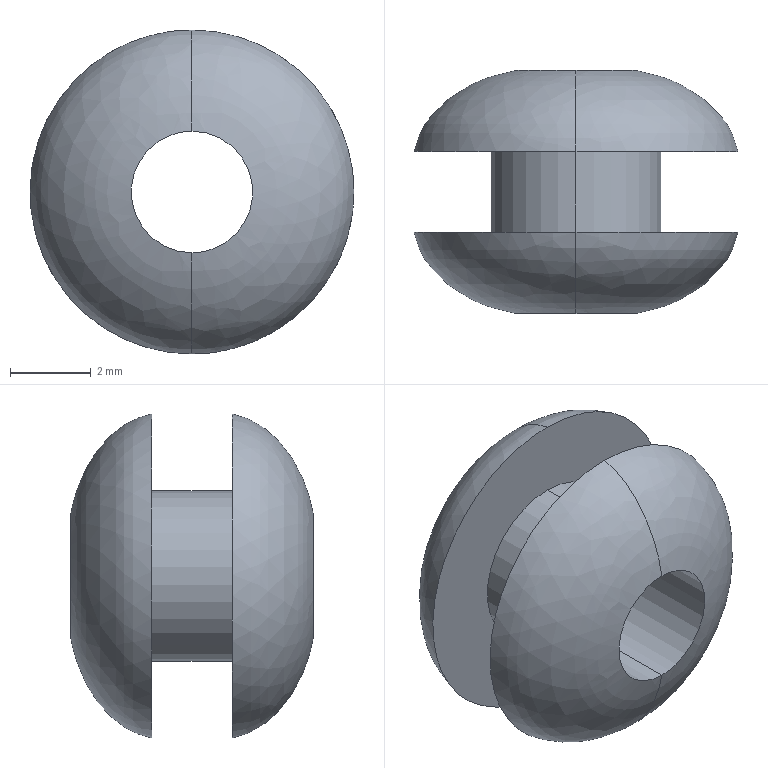Part | SolidWorks | features BaseBody 1 | 1 solid | 10 faces | box 8 x 6 x 8 mm | volume 125.45 mm3 | spline 4 | cylinder 4 | plane 2 | commonest cylinder face diameters 3 x2 4.2 x2
STEP:
#1=CARTESIAN_POINT('',(0.,-1.,-4.));
#2=VERTEX_POINT('',#1);
#3=CARTESIAN_POINT('',(0.,-3.,-1.5));
#4=VERTEX_POINT('',#3);
#5=CARTESIAN_POINT('',(0.,-1.,-4.));
#6=CARTESIAN_POINT('',(0.,-2.617,-3.692));
#7=CARTESIAN_POINT('',(0.,-3.,-1.5));
#8=(BOUNDED_CURVE()B_SPLINE_CURVE(2,(#5,#6,#7),.UNSPECIFIED.,.F.,.F.)B_SPLINE_CURVE_WITH_KNOTS((3,3),(0.,1.),.UNSPECIFIED.)CURVE()GEOMETRIC_REPRESENTATION_ITEM()RATIONAL_B_SPLINE_CURVE((1.,0.8226,1.))REPRESENTATION_ITEM(''));
#9=EDGE_CURVE('',#2,#4,#8,.T.);
#10=ORIENTED_EDGE('',*,*,#9,.F.);
#11=CARTESIAN_POINT('',(0.,-1.,4.));
#12=VERTEX_POINT('',#11);
#13=CARTESIAN_POINT('',(0.,-1.,4.));
#14=CARTESIAN_POINT('',(0.5299,-1.,4.));
#15=CARTESIAN_POINT('',(1.042,-1.,3.898));
#16=CARTESIAN_POINT('',(2.02,-1.,3.493));
#17=CARTESIAN_POINT('',(2.454,-1.,3.203));
#18=CARTESIAN_POINT('',(3.203,-1.,2.454));
#19=CARTESIAN_POINT('',(3.493,-1.,2.02));
#20=CARTESIAN_POINT('',(3.898,-1.,1.042));
#21=CARTESIAN_POINT('',(4.,-1.,0.5294));
#22=CARTESIAN_POINT('',(4.,-1.,-0.5294));
#23=CARTESIAN_POINT('',(3.898,-1.,-1.042));
#24=CARTESIAN_POINT('',(3.493,-1.,-2.02));
#25=CARTESIAN_POINT('',(3.203,-1.,-2.454));
#26=CARTESIAN_POINT('',(2.454,-1.,-3.203));
#27=CARTESIAN_POINT('',(2.02,-1.,-3.493));
#28=CARTESIAN_POINT('',(1.041,-1.,-3.898));
#29=CARTESIAN_POINT('',(0.5312,-1.,-4.));
#30=CARTESIAN_POINT('',(0.,-1.,-4.));
#31=B_SPLINE_CURVE_WITH_KNOTS('',3,(#13,#14,#15,#16,#17,#18,#19,#20,#21,#22,#23,#24,#25,#26,#27,#28,#29,#30),.UNSPECIFIED.,.F.,.F.,(4,2,2,2,2,2,2,2,4),(0.,0.125,0.25,0.375,0.5,0.625,0.75,0.875,1.),.UNSPECIFIED.);
#32=EDGE_CURVE('',#12,#2,#31,.T.);
#33=ORIENTED_EDGE('',*,*,#32,.F.);
#34=CARTESIAN_POINT('',(0.,-3.,1.5));
#35=VERTEX_POINT('',#34);
#36=CARTESIAN_POINT('',(0.,-1.,4.));
#37=CARTESIAN_POINT('',(0.,-2.617,3.692));
#38=CARTESIAN_POINT('',(0.,-3.,1.5));
#39=(BOUNDED_CURVE()B_SPLINE_CURVE(2,(#36,#37,#38),.UNSPECIFIED.,.F.,.F.)B_SPLINE_CURVE_WITH_KNOTS((3,3),(0.,1.),.UNSPECIFIED.)CURVE()GEOMETRIC_REPRESENTATION_ITEM()RATIONAL_B_SPLINE_CURVE((1.,0.8226,1.))REPRESENTATION_ITEM(''));
#40=EDGE_CURVE('',#12,#35,#39,.T.);
#41=ORIENTED_EDGE('',*,*,#40,.T.);
#42=CARTESIAN_POINT('',(0.,-3.,1.5));
#43=CARTESIAN_POINT('',(0.1963,-3.,1.5));
#44=CARTESIAN_POINT('',(0.3926,-3.,1.461));
#45=CARTESIAN_POINT('',(0.7554,-3.,1.311));
#46=CARTESIAN_POINT('',(0.9218,-3.,1.2));
#47=CARTESIAN_POINT('',(1.2,-3.,0.9218));
#48=CARTESIAN_POINT('',(1.311,-3.,0.7554));
#49=CARTESIAN_POINT('',(1.461,-3.,0.3926));
#50=CARTESIAN_POINT('',(1.5,-3.,0.1963));
#51=CARTESIAN_POINT('',(1.5,-3.,-0.1963));
#52=CARTESIAN_POINT('',(1.461,-3.,-0.3926));
#53=CARTESIAN_POINT('',(1.311,-3.,-0.7554));
#54=CARTESIAN_POINT('',(1.2,-3.,-0.9218));
#55=CARTESIAN_POINT('',(0.9218,-3.,-1.2));
#56=CARTESIAN_POINT('',(0.7554,-3.,-1.311));
#57=CARTESIAN_POINT('',(0.3926,-3.,-1.461));
#58=CARTESIAN_POINT('',(0.1963,-3.,-1.5));
#59=CARTESIAN_POINT('',(0.,-3.,-1.5));
#60=B_SPLINE_CURVE_WITH_KNOTS('',3,(#42,#43,#44,#45,#46,#47,#48,#49,#50,#51,#52,#53,#54,#55,#56,#57,#58,#59),.UNSPECIFIED.,.F.,.F.,(4,2,2,2,2,2,2,2,4),(0.,0.125,0.25,0.375,0.5,0.625,0.75,0.875,1.),.UNSPECIFIED.);
#61=EDGE_CURVE('',#35,#4,#60,.T.);
#62=ORIENTED_EDGE('',*,*,#61,.T.);
#63=EDGE_LOOP('',(#10,#33,#41,#62));
#64=FACE_OUTER_BOUND('',#63,.T.);
#65=CARTESIAN_POINT('',(0.,-1.,4.));
#66=CARTESIAN_POINT('',(0.5236,-1.,4.));
#67=CARTESIAN_POINT('',(1.047,-1.,3.896));
#68=CARTESIAN_POINT('',(2.014,-1.,3.495));
#69=CARTESIAN_POINT('',(2.458,-1.,3.199));
#70=CARTESIAN_POINT('',(3.199,-1.,2.458));
#71=CARTESIAN_POINT('',(3.495,-1.,2.014));
#72=CARTESIAN_POINT('',(3.896,-1.,1.047));
#73=CARTESIAN_POINT('',(4.,-1.,0.5236));
#74=CARTESIAN_POINT('',(4.,-1.,-0.5236));
#75=CARTESIAN_POINT('',(3.896,-1.,-1.047));
#76=CARTESIAN_POINT('',(3.495,-1.,-2.014));
#77=CARTESIAN_POINT('',(3.199,-1.,-2.458));
#78=CARTESIAN_POINT('',(2.458,-1.,-3.199));
#79=CARTESIAN_POINT('',(2.014,-1.,-3.495));
#80=CARTESIAN_POINT('',(1.047,-1.,-3.896));
#81=CARTESIAN_POINT('',(0.5236,-1.,-4.));
#82=CARTESIAN_POINT('',(-0.5236,-1.,-4.));
#83=CARTESIAN_POINT('',(-1.047,-1.,-3.896));
#84=CARTESIAN_POINT('',(-2.014,-1.,-3.495));
#85=CARTESIAN_POINT('',(-2.458,-1.,-3.199));
#86=CARTESIAN_POINT('',(-3.199,-1.,-2.458));
#87=CARTESIAN_POINT('',(-3.495,-1.,-2.014));
#88=CARTESIAN_POINT('',(-3.896,-1.,-1.047));
#89=CARTESIAN_POINT('',(-4.,-1.,-0.5236));
#90=CARTESIAN_POINT('',(-4.,-1.,0.5236));
#91=CARTESIAN_POINT('',(-3.896,-1.,1.047));
#92=CARTESIAN_POINT('',(-3.495,-1.,2.014));
#93=CARTESIAN_POINT('',(-3.199,-1.,2.458));
#94=CARTESIAN_POINT('',(-2.458,-1.,3.199));
#95=CARTESIAN_POINT('',(-2.014,-1.,3.495));
#96=CARTESIAN_POINT('',(-1.047,-1.,3.896));
#97=CARTESIAN_POINT('',(-0.5236,-1.,4.));
#98=CARTESIAN_POINT('',(0.,-1.,4.));
#99=CARTESIAN_POINT('',(0.,-2.617,3.692));
#100=CARTESIAN_POINT('',(0.4833,-2.617,3.692));
#101=CARTESIAN_POINT('',(0.9664,-2.617,3.596));
#102=CARTESIAN_POINT('',(1.859,-2.617,3.226));
#103=CARTESIAN_POINT('',(2.269,-2.617,2.952));
#104=CARTESIAN_POINT('',(2.952,-2.617,2.269));
#105=CARTESIAN_POINT('',(3.226,-2.617,1.859));
#106=CARTESIAN_POINT('',(3.596,-2.617,0.9664));
#107=CARTESIAN_POINT('',(3.692,-2.617,0.4833));
#108=CARTESIAN_POINT('',(3.692,-2.617,-0.4833));
#109=CARTESIAN_POINT('',(3.596,-2.617,-0.9664));
#110=CARTESIAN_POINT('',(3.226,-2.617,-1.859));
#111=CARTESIAN_POINT('',(2.952,-2.617,-2.269));
#112=CARTESIAN_POINT('',(2.269,-2.617,-2.952));
#113=CARTESIAN_POINT('',(1.859,-2.617,-3.226));
#114=CARTESIAN_POINT('',(0.9664,-2.617,-3.596));
#115=CARTESIAN_POINT('',(0.4833,-2.617,-3.692));
#116=CARTESIAN_POINT('',(-0.4833,-2.617,-3.692));
#117=CARTESIAN_POINT('',(-0.9664,-2.617,-3.596));
#118=CARTESIAN_POINT('',(-1.859,-2.617,-3.226));
#119=CARTESIAN_POINT('',(-2.269,-2.617,-2.952));
#120=CARTESIAN_POINT('',(-2.952,-2.617,-2.269));
#121=CARTESIAN_POINT('',(-3.226,-2.617,-1.859));
#122=CARTESIAN_POINT('',(-3.596,-2.617,-0.9664));
#123=CARTESIAN_POINT('',(-3.692,-2.617,-0.4833));
#124=CARTESIAN_POINT('',(-3.692,-2.617,0.4833));
#125=CARTESIAN_POINT('',(-3.596,-2.617,0.9664));
#126=CARTESIAN_POINT('',(-3.226,-2.617,1.859));
#127=CARTESIAN_POINT('',(-2.952,-2.617,2.269));
#128=CARTESIAN_POINT('',(-2.269,-2.617,2.952));
#129=CARTESIAN_POINT('',(-1.859,-2.617,3.226));
#130=CARTESIAN_POINT('',(-0.9664,-2.617,3.596));
#131=CARTESIAN_POINT('',(-0.4833,-2.617,3.692));
#132=CARTESIAN_POINT('',(0.,-2.617,3.692));
#133=CARTESIAN_POINT('',(0.,-3.,1.5));
#134=CARTESIAN_POINT('',(0.1963,-3.,1.5));
#135=CARTESIAN_POINT('',(0.3926,-3.,1.461));
#136=CARTESIAN_POINT('',(0.7554,-3.,1.311));
#137=CARTESIAN_POINT('',(0.9218,-3.,1.2));
#138=CARTESIAN_POINT('',(1.2,-3.,0.9218));
#139=CARTESIAN_POINT('',(1.311,-3.,0.7554));
#140=CARTESIAN_POINT('',(1.461,-3.,0.3926));
#141=CARTESIAN_POINT('',(1.5,-3.,0.1963));
#142=CARTESIAN_POINT('',(1.5,-3.,-0.1963));
#143=CARTESIAN_POINT('',(1.461,-3.,-0.3926));
#144=CARTESIAN_POINT('',(1.311,-3.,-0.7554));
#145=CARTESIAN_POINT('',(1.2,-3.,-0.9218));
#146=CARTESIAN_POINT('',(0.9218,-3.,-1.2));
#147=CARTESIAN_POINT('',(0.7554,-3.,-1.311));
#148=CARTESIAN_POINT('',(0.3926,-3.,-1.461));
#149=CARTESIAN_POINT('',(0.1963,-3.,-1.5));
#150=CARTESIAN_POINT('',(-0.1963,-3.,-1.5));
#151=CARTESIAN_POINT('',(-0.3926,-3.,-1.461));
#152=CARTESIAN_POINT('',(-0.7554,-3.,-1.311));
#153=CARTESIAN_POINT('',(-0.9218,-3.,-1.2));
#154=CARTESIAN_POINT('',(-1.2,-3.,-0.9218));
#155=CARTESIAN_POINT('',(-1.311,-3.,-0.7554));
#156=CARTESIAN_POINT('',(-1.461,-3.,-0.3926));
#157=CARTESIAN_POINT('',(-1.5,-3.,-0.1963));
#158=CARTESIAN_POINT('',(-1.5,-3.,0.1963));
#159=CARTESIAN_POINT('',(-1.461,-3.,0.3926));
#160=CARTESIAN_POINT('',(-1.311,-3.,0.7554));
#161=CARTESIAN_POINT('',(-1.2,-3.,0.9218));
#162=CARTESIAN_POINT('',(-0.9218,-3.,1.2));
#163=CARTESIAN_POINT('',(-0.7554,-3.,1.311));
#164=CARTESIAN_POINT('',(-0.3926,-3.,1.461));
#165=CARTESIAN_POINT('',(-0.1963,-3.,1.5));
#166=CARTESIAN_POINT('',(0.,-3.,1.5));
#167=(BOUNDED_SURFACE()B_SPLINE_SURFACE(2,3,((#65,#66,#67,#68,#69,#70,#71,#72,#73,#74,#75,#76,#77,#78,#79,#80,#81,#82,#83,#84,#85,#86,#87,#88,#89,#90,#91,#92,#93,#94,#95,#96,#97,#98),(#99,#100,#101,#102,#103,#104,#105,#106,#107,#108,#109,#110,#111,#112,#113,#114,#115,#116,#117,#118,#119,#120,#121,#122,#123,#124,#125,#126,#127,#128,#129,#130,#131,#132),(#133,#134,#135,#136,#137,#138,#139,#140,#141,#142,#143,#144,#145,#146,#147,#148,#149,#150,#151,#152,#153,#154,#155,#156,#157,#158,#159,#160,#161,#162,#163,#164,#165,#166)),.UNSPECIFIED.,.F.,.T.,.F.)B_SPLINE_SURFACE_WITH_KNOTS((3,3),(4,2,2,2,2,2,2,2,2,2,2,2,2,2,2,2,4),(0.,1.),(0.,0.3927,0.7854,1.178,1.571,1.963,2.356,2.749,3.142,3.534,3.927,4.32,4.712,5.105,5.498,5.89,6.283),.UNSPECIFIED.)GEOMETRIC_REPRESENTATION_ITEM()RATIONAL_B_SPLINE_SURFACE(((1.,1.,1.,1.,1.,1.,1.,1.,1.,1.,1.,1.,1.,1.,1.,1.,1.,1.,1.,1.,1.,1.,1.,1.,1.,1.,1.,1.,1.,1.,1.,1.,1.,1.),(0.8226,0.8226,0.8226,0.8226,0.8226,0.8226,0.8226,0.8226,0.8226,0.8226,0.8226,0.8226,0.8226,0.8226,0.8226,0.8226,0.8226,0.8226,0.8226,0.8226,0.8226,0.8226,0.8226,0.8226,0.8226,0.8226,0.8226,0.8226,0.8226,0.8226,0.8226,0.8226,0.8226,0.8226),(1.,1.,1.,1.,1.,1.,1.,1.,1.,1.,1.,1.,1.,1.,1.,1.,1.,1.,1.,1.,1.,1.,1.,1.,1.,1.,1.,1.,1.,1.,1.,1.,1.,1.)))REPRESENTATION_ITEM('')SURFACE());
#168=ADVANCED_FACE('',(#64),#167,.T.);
#169=CARTESIAN_POINT('',(0.,-1.,-2.1));
#170=VERTEX_POINT('',#169);
#171=CARTESIAN_POINT('',(0.,-1.,2.1));
#172=VERTEX_POINT('',#171);
#173=CARTESIAN_POINT('',(0.,-1.,0.));
#174=DIRECTION('',(0.,1.,0.));
#175=DIRECTION('',(0.,0.,1.));
#176=AXIS2_PLACEMENT_3D('',#173,#174,#175);
#177=CIRCLE('',#176,2.1);
#178=EDGE_CURVE('',#170,#172,#177,.T.);
#179=ORIENTED_EDGE('',*,*,#178,.F.);
#180=CARTESIAN_POINT('',(0.,-1.,0.));
#181=DIRECTION('',(0.,1.,0.));
#182=DIRECTION('',(0.,0.,1.));
#183=AXIS2_PLACEMENT_3D('',#180,#181,#182);
#184=CIRCLE('',#183,2.1);
#185=EDGE_CURVE('',#172,#170,#184,.T.);
#186=ORIENTED_EDGE('',*,*,#185,.F.);
#187=EDGE_LOOP('',(#179,#186));
#188=FACE_BOUND('',#187,.T.);
#189=ORIENTED_EDGE('',*,*,#32,.T.);
#190=CARTESIAN_POINT('',(0.,-1.,-4.));
#191=CARTESIAN_POINT('',(-0.5297,-1.,-4.));
#192=CARTESIAN_POINT('',(-1.042,-1.,-3.898));
#193=CARTESIAN_POINT('',(-2.02,-1.,-3.493));
#194=CARTESIAN_POINT('',(-2.454,-1.,-3.203));
#195=CARTESIAN_POINT('',(-3.203,-1.,-2.454));
#196=CARTESIAN_POINT('',(-3.493,-1.,-2.02));
#197=CARTESIAN_POINT('',(-3.898,-1.,-1.042));
#198=CARTESIAN_POINT('',(-4.,-1.,-0.5293));
#199=CARTESIAN_POINT('',(-4.,-1.,0.5293));
#200=CARTESIAN_POINT('',(-3.898,-1.,1.042));
#201=CARTESIAN_POINT('',(-3.493,-1.,2.02));
#202=CARTESIAN_POINT('',(-3.203,-1.,2.454));
#203=CARTESIAN_POINT('',(-2.454,-1.,3.203));
#204=CARTESIAN_POINT('',(-2.02,-1.,3.493));
#205=CARTESIAN_POINT('',(-1.041,-1.,3.899));
#206=CARTESIAN_POINT('',(-0.531,-1.,4.));
#207=CARTESIAN_POINT('',(0.,-1.,4.));
#208=B_SPLINE_CURVE_WITH_KNOTS('',3,(#190,#191,#192,#193,#194,#195,#196,#197,#198,#199,#200,#201,#202,#203,#204,#205,#206,#207),.UNSPECIFIED.,.F.,.F.,(4,2,2,2,2,2,2,2,4),(0.,0.125,0.25,0.375,0.5,0.625,0.75,0.875,1.),.UNSPECIFIED.);
#209=EDGE_CURVE('',#2,#12,#208,.T.);
#210=ORIENTED_EDGE('',*,*,#209,.T.);
#211=EDGE_LOOP('',(#189,#210));
#212=FACE_OUTER_BOUND('',#211,.T.);
#213=CARTESIAN_POINT('',(0.,-1.,0.));
#214=DIRECTION('',(0.,-1.,0.));
#215=DIRECTION('',(0.,0.,-1.));
#216=AXIS2_PLACEMENT_3D('',#213,#214,#215);
#217=PLANE('',#216);
#218=ADVANCED_FACE('',(#188,#212),#217,.F.);
#219=CARTESIAN_POINT('',(0.,3.,-1.5));
#220=VERTEX_POINT('',#219);
#221=CARTESIAN_POINT('',(0.,1.,-4.));
#222=VERTEX_POINT('',#221);
#223=CARTESIAN_POINT('',(0.,3.,-1.5));
#224=CARTESIAN_POINT('',(0.,2.617,-3.692));
#225=CARTESIAN_POINT('',(0.,1.,-4.));
#226=(BOUNDED_CURVE()B_SPLINE_CURVE(2,(#223,#224,#225),.UNSPECIFIED.,.F.,.F.)B_SPLINE_CURVE_WITH_KNOTS((3,3),(0.,1.),.UNSPECIFIED.)CURVE()GEOMETRIC_REPRESENTATION_ITEM()RATIONAL_B_SPLINE_CURVE((1.,0.8226,1.))REPRESENTATION_ITEM(''));
#227=EDGE_CURVE('',#220,#222,#226,.T.);
#228=ORIENTED_EDGE('',*,*,#227,.F.);
#229=CARTESIAN_POINT('',(0.,3.,1.5));
#230=VERTEX_POINT('',#229);
#231=CARTESIAN_POINT('',(0.,3.,1.5));
#232=CARTESIAN_POINT('',(0.1963,3.,1.5));
#233=CARTESIAN_POINT('',(0.3926,3.,1.461));
#234=CARTESIAN_POINT('',(0.7554,3.,1.311));
#235=CARTESIAN_POINT('',(0.9218,3.,1.2));
#236=CARTESIAN_POINT('',(1.2,3.,0.9218));
#237=CARTESIAN_POINT('',(1.311,3.,0.7554));
#238=CARTESIAN_POINT('',(1.461,3.,0.3926));
#239=CARTESIAN_POINT('',(1.5,3.,0.1963));
#240=CARTESIAN_POINT('',(1.5,3.,-0.1963));
#241=CARTESIAN_POINT('',(1.461,3.,-0.3926));
#242=CARTESIAN_POINT('',(1.311,3.,-0.7554));
#243=CARTESIAN_POINT('',(1.2,3.,-0.9218));
#244=CARTESIAN_POINT('',(0.9218,3.,-1.2));
#245=CARTESIAN_POINT('',(0.7554,3.,-1.311));
#246=CARTESIAN_POINT('',(0.3926,3.,-1.461));
#247=CARTESIAN_POINT('',(0.1963,3.,-1.5));
#248=CARTESIAN_POINT('',(0.,3.,-1.5));
#249=B_SPLINE_CURVE_WITH_KNOTS('',3,(#231,#232,#233,#234,#235,#236,#237,#238,#239,#240,#241,#242,#243,#244,#245,#246,#247,#248),.UNSPECIFIED.,.F.,.F.,(4,2,2,2,2,2,2,2,4),(0.,0.125,0.25,0.375,0.5,0.625,0.75,0.875,1.),.UNSPECIFIED.);
#250=EDGE_CURVE('',#230,#220,#249,.T.);
#251=ORIENTED_EDGE('',*,*,#250,.F.);
#252=CARTESIAN_POINT('',(0.,1.,4.));
#253=VERTEX_POINT('',#252);
#254=CARTESIAN_POINT('',(0.,3.,1.5));
#255=CARTESIAN_POINT('',(0.,2.617,3.692));
#256=CARTESIAN_POINT('',(0.,1.,4.));
#257=(BOUNDED_CURVE()B_SPLINE_CURVE(2,(#254,#255,#256),.UNSPECIFIED.,.F.,.F.)B_SPLINE_CURVE_WITH_KNOTS((3,3),(0.,1.),.UNSPECIFIED.)CURVE()GEOMETRIC_REPRESENTATION_ITEM()RATIONAL_B_SPLINE_CURVE((1.,0.8226,1.))REPRESENTATION_ITEM(''));
#258=EDGE_CURVE('',#230,#253,#257,.T.);
#259=ORIENTED_EDGE('',*,*,#258,.T.);
#260=CARTESIAN_POINT('',(0.,1.,4.));
#261=CARTESIAN_POINT('',(0.5236,1.,4.));
#262=CARTESIAN_POINT('',(1.047,1.,3.896));
#263=CARTESIAN_POINT('',(2.014,1.,3.495));
#264=CARTESIAN_POINT('',(2.458,1.,3.199));
#265=CARTESIAN_POINT('',(3.199,1.,2.458));
#266=CARTESIAN_POINT('',(3.495,1.,2.014));
#267=CARTESIAN_POINT('',(3.896,1.,1.047));
#268=CARTESIAN_POINT('',(4.,1.,0.5236));
#269=CARTESIAN_POINT('',(4.,1.,-0.5236));
#270=CARTESIAN_POINT('',(3.896,1.,-1.047));
#271=CARTESIAN_POINT('',(3.495,1.,-2.014));
#272=CARTESIAN_POINT('',(3.199,1.,-2.458));
#273=CARTESIAN_POINT('',(2.458,1.,-3.199));
#274=CARTESIAN_POINT('',(2.014,1.,-3.495));
#275=CARTESIAN_POINT('',(1.047,1.,-3.896));
#276=CARTESIAN_POINT('',(0.5236,1.,-4.));
#277=CARTESIAN_POINT('',(0.,1.,-4.));
#278=B_SPLINE_CURVE_WITH_KNOTS('',3,(#260,#261,#262,#263,#264,#265,#266,#267,#268,#269,#270,#271,#272,#273,#274,#275,#276,#277),.UNSPECIFIED.,.F.,.F.,(4,2,2,2,2,2,2,2,4),(0.,0.0625,0.125,0.1875,0.25,0.3125,0.375,0.4375,0.5),.UNSPECIFIED.);
#279=EDGE_CURVE('',#253,#222,#278,.T.);
#280=ORIENTED_EDGE('',*,*,#279,.T.);
#281=EDGE_LOOP('',(#228,#251,#259,#280));
#282=FACE_OUTER_BOUND('',#281,.T.);
#283=CARTESIAN_POINT('',(0.,3.,1.5));
#284=CARTESIAN_POINT('',(0.1963,3.,1.5));
#285=CARTESIAN_POINT('',(0.3926,3.,1.461));
#286=CARTESIAN_POINT('',(0.7554,3.,1.311));
#287=CARTESIAN_POINT('',(0.9218,3.,1.2));
#288=CARTESIAN_POINT('',(1.2,3.,0.9218));
#289=CARTESIAN_POINT('',(1.311,3.,0.7554));
#290=CARTESIAN_POINT('',(1.461,3.,0.3926));
#291=CARTESIAN_POINT('',(1.5,3.,0.1963));
#292=CARTESIAN_POINT('',(1.5,3.,-0.1963));
#293=CARTESIAN_POINT('',(1.461,3.,-0.3926));
#294=CARTESIAN_POINT('',(1.311,3.,-0.7554));
#295=CARTESIAN_POINT('',(1.2,3.,-0.9218));
#296=CARTESIAN_POINT('',(0.9218,3.,-1.2));
#297=CARTESIAN_POINT('',(0.7554,3.,-1.311));
#298=CARTESIAN_POINT('',(0.3926,3.,-1.461));
#299=CARTESIAN_POINT('',(0.1963,3.,-1.5));
#300=CARTESIAN_POINT('',(0.,3.,-1.5));
#301=CARTESIAN_POINT('',(0.,2.617,3.692));
#302=CARTESIAN_POINT('',(0.4833,2.617,3.692));
#303=CARTESIAN_POINT('',(0.9664,2.617,3.596));
#304=CARTESIAN_POINT('',(1.859,2.617,3.226));
#305=CARTESIAN_POINT('',(2.269,2.617,2.952));
#306=CARTESIAN_POINT('',(2.952,2.617,2.269));
#307=CARTESIAN_POINT('',(3.226,2.617,1.859));
#308=CARTESIAN_POINT('',(3.596,2.617,0.9664));
#309=CARTESIAN_POINT('',(3.692,2.617,0.4833));
#310=CARTESIAN_POINT('',(3.692,2.617,-0.4833));
#311=CARTESIAN_POINT('',(3.596,2.617,-0.9664));
#312=CARTESIAN_POINT('',(3.226,2.617,-1.859));
#313=CARTESIAN_POINT('',(2.952,2.617,-2.269));
#314=CARTESIAN_POINT('',(2.269,2.617,-2.952));
#315=CARTESIAN_POINT('',(1.859,2.617,-3.226));
#316=CARTESIAN_POINT('',(0.9664,2.617,-3.596));
#317=CARTESIAN_POINT('',(0.4833,2.617,-3.692));
#318=CARTESIAN_POINT('',(0.,2.617,-3.692));
#319=CARTESIAN_POINT('',(0.,1.,4.));
#320=CARTESIAN_POINT('',(0.5236,1.,4.));
#321=CARTESIAN_POINT('',(1.047,1.,3.896));
#322=CARTESIAN_POINT('',(2.014,1.,3.495));
#323=CARTESIAN_POINT('',(2.458,1.,3.199));
#324=CARTESIAN_POINT('',(3.199,1.,2.458));
#325=CARTESIAN_POINT('',(3.495,1.,2.014));
#326=CARTESIAN_POINT('',(3.896,1.,1.047));
#327=CARTESIAN_POINT('',(4.,1.,0.5236));
#328=CARTESIAN_POINT('',(4.,1.,-0.5236));
#329=CARTESIAN_POINT('',(3.896,1.,-1.047));
#330=CARTESIAN_POINT('',(3.495,1.,-2.014));
#331=CARTESIAN_POINT('',(3.199,1.,-2.458));
#332=CARTESIAN_POINT('',(2.458,1.,-3.199));
#333=CARTESIAN_POINT('',(2.014,1.,-3.495));
#334=CARTESIAN_POINT('',(1.047,1.,-3.896));
#335=CARTESIAN_POINT('',(0.5236,1.,-4.));
#336=CARTESIAN_POINT('',(0.,1.,-4.));
#337=(BOUNDED_SURFACE()B_SPLINE_SURFACE(2,3,((#283,#284,#285,#286,#287,#288,#289,#290,#291,#292,#293,#294,#295,#296,#297,#298,#299,#300),(#301,#302,#303,#304,#305,#306,#307,#308,#309,#310,#311,#312,#313,#314,#315,#316,#317,#318),(#319,#320,#321,#322,#323,#324,#325,#326,#327,#328,#329,#330,#331,#332,#333,#334,#335,#336)),.UNSPECIFIED.,.F.,.F.,.T.)B_SPLINE_SURFACE_WITH_KNOTS((3,3),(4,2,2,2,2,2,2,2,4),(0.,1.),(0.,0.3927,0.7854,1.178,1.571,1.963,2.356,2.749,3.142),.UNSPECIFIED.)GEOMETRIC_REPRESENTATION_ITEM()RATIONAL_B_SPLINE_SURFACE(((1.,1.,1.,1.,1.,1.,1.,1.,1.,1.,1.,1.,1.,1.,1.,1.,1.,1.),(0.8226,0.8226,0.8226,0.8226,0.8226,0.8226,0.8226,0.8226,0.8226,0.8226,0.8226,0.8226,0.8226,0.8226,0.8226,0.8226,0.8226,0.8226),(1.,1.,1.,1.,1.,1.,1.,1.,1.,1.,1.,1.,1.,1.,1.,1.,1.,1.)))REPRESENTATION_ITEM('')SURFACE());
#338=ADVANCED_FACE('',(#282),#337,.T.);
#339=CARTESIAN_POINT('',(0.,1.,-2.1));
#340=VERTEX_POINT('',#339);
#341=CARTESIAN_POINT('',(0.,1.,2.1));
#342=VERTEX_POINT('',#341);
#343=CARTESIAN_POINT('',(0.,1.,0.));
#344=DIRECTION('',(0.,1.,0.));
#345=DIRECTION('',(0.,0.,1.));
#346=AXIS2_PLACEMENT_3D('',#343,#344,#345);
#347=CIRCLE('',#346,2.1);
#348=EDGE_CURVE('',#340,#342,#347,.T.);
#349=ORIENTED_EDGE('',*,*,#348,.T.);
#350=CARTESIAN_POINT('',(0.,1.,0.));
#351=DIRECTION('',(0.,1.,0.));
#352=DIRECTION('',(0.,0.,1.));
#353=AXIS2_PLACEMENT_3D('',#350,#351,#352);
#354=CIRCLE('',#353,2.1);
#355=EDGE_CURVE('',#342,#340,#354,.T.);
#356=ORIENTED_EDGE('',*,*,#355,.T.);
#357=EDGE_LOOP('',(#349,#356));
#358=FACE_BOUND('',#357,.T.);
#359=ORIENTED_EDGE('',*,*,#279,.F.);
#360=CARTESIAN_POINT('',(0.,1.,-4.));
#361=CARTESIAN_POINT('',(-0.5236,1.,-4.));
#362=CARTESIAN_POINT('',(-1.047,1.,-3.896));
#363=CARTESIAN_POINT('',(-2.014,1.,-3.495));
#364=CARTESIAN_POINT('',(-2.458,1.,-3.199));
#365=CARTESIAN_POINT('',(-3.199,1.,-2.458));
#366=CARTESIAN_POINT('',(-3.495,1.,-2.014));
#367=CARTESIAN_POINT('',(-3.896,1.,-1.047));
#368=CARTESIAN_POINT('',(-4.,1.,-0.5236));
#369=CARTESIAN_POINT('',(-4.,1.,0.5236));
#370=CARTESIAN_POINT('',(-3.896,1.,1.047));
#371=CARTESIAN_POINT('',(-3.495,1.,2.014));
#372=CARTESIAN_POINT('',(-3.199,1.,2.458));
#373=CARTESIAN_POINT('',(-2.458,1.,3.199));
#374=CARTESIAN_POINT('',(-2.014,1.,3.495));
#375=CARTESIAN_POINT('',(-1.047,1.,3.896));
#376=CARTESIAN_POINT('',(-0.5236,1.,4.));
#377=CARTESIAN_POINT('',(0.,1.,4.));
#378=B_SPLINE_CURVE_WITH_KNOTS('',3,(#360,#361,#362,#363,#364,#365,#366,#367,#368,#369,#370,#371,#372,#373,#374,#375,#376,#377),.UNSPECIFIED.,.F.,.F.,(4,2,2,2,2,2,2,2,4),(0.5,0.5625,0.625,0.6875,0.75,0.8125,0.875,0.9375,1.),.UNSPECIFIED.);
#379=EDGE_CURVE('',#222,#253,#378,.T.);
#380=ORIENTED_EDGE('',*,*,#379,.F.);
#381=EDGE_LOOP('',(#359,#380));
#382=FACE_OUTER_BOUND('',#381,.T.);
#383=CARTESIAN_POINT('',(0.,1.,0.));
#384=DIRECTION('',(0.,1.,0.));
#385=DIRECTION('',(1.,0.,0.));
#386=AXIS2_PLACEMENT_3D('',#383,#384,#385);
#387=PLANE('',#386);
#388=ADVANCED_FACE('',(#358,#382),#387,.F.);
#389=CARTESIAN_POINT('',(0.,1.,1.5));
#390=DIRECTION('',(0.,-1.,0.));
#391=VECTOR('',#390,1000.);
#392=LINE('',#389,#391);
#393=EDGE_CURVE('',#230,#35,#392,.T.);
#394=ORIENTED_EDGE('',*,*,#393,.F.);
#395=ORIENTED_EDGE('',*,*,#250,.T.);
#396=CARTESIAN_POINT('',(0.,1.,-1.5));
#397=DIRECTION('',(0.,-1.,0.));
#398=VECTOR('',#397,1000.);
#399=LINE('',#396,#398);
#400=EDGE_CURVE('',#220,#4,#399,.T.);
#401=ORIENTED_EDGE('',*,*,#400,.T.);
#402=ORIENTED_EDGE('',*,*,#61,.F.);
#403=EDGE_LOOP('',(#394,#395,#401,#402));
#404=FACE_OUTER_BOUND('',#403,.T.);
#405=CARTESIAN_POINT('',(0.,1.,0.));
#406=DIRECTION('',(0.,-1.,0.));
#407=DIRECTION('',(0.,0.,-1.));
#408=AXIS2_PLACEMENT_3D('',#405,#406,#407);
#409=CYLINDRICAL_SURFACE('',#408,1.5);
#410=ADVANCED_FACE('',(#404),#409,.F.);
#411=CARTESIAN_POINT('',(0.,1.,2.1));
#412=DIRECTION('',(0.,-1.,0.));
#413=VECTOR('',#412,1000.);
#414=LINE('',#411,#413);
#415=EDGE_CURVE('',#342,#172,#414,.T.);
#416=ORIENTED_EDGE('',*,*,#415,.F.);
#417=ORIENTED_EDGE('',*,*,#348,.F.);
#418=CARTESIAN_POINT('',(0.,1.,-2.1));
#419=DIRECTION('',(0.,-1.,0.));
#420=VECTOR('',#419,1000.);
#421=LINE('',#418,#420);
#422=EDGE_CURVE('',#340,#170,#421,.T.);
#423=ORIENTED_EDGE('',*,*,#422,.T.);
#424=ORIENTED_EDGE('',*,*,#178,.T.);
#425=EDGE_LOOP('',(#416,#417,#423,#424));
#426=FACE_OUTER_BOUND('',#425,.T.);
#427=CARTESIAN_POINT('',(0.,1.,0.));
#428=DIRECTION('',(0.,-1.,0.));
#429=DIRECTION('',(0.,0.,-1.));
#430=AXIS2_PLACEMENT_3D('',#427,#428,#429);
#431=CYLINDRICAL_SURFACE('',#430,2.1);
#432=ADVANCED_FACE('',(#426),#431,.T.);
#433=ORIENTED_EDGE('',*,*,#355,.F.);
#434=ORIENTED_EDGE('',*,*,#415,.T.);
#435=ORIENTED_EDGE('',*,*,#185,.T.);
#436=ORIENTED_EDGE('',*,*,#422,.F.);
#437=EDGE_LOOP('',(#433,#434,#435,#436));
#438=FACE_OUTER_BOUND('',#437,.T.);
#439=CARTESIAN_POINT('',(0.,1.,0.));
#440=DIRECTION('',(0.,-1.,0.));
#441=DIRECTION('',(0.,0.,-1.));
#442=AXIS2_PLACEMENT_3D('',#439,#440,#441);
#443=CYLINDRICAL_SURFACE('',#442,2.1);
#444=ADVANCED_FACE('',(#438),#443,.T.);
#445=CARTESIAN_POINT('',(0.,3.,-1.5));
#446=CARTESIAN_POINT('',(-0.1963,3.,-1.5));
#447=CARTESIAN_POINT('',(-0.3926,3.,-1.461));
#448=CARTESIAN_POINT('',(-0.7554,3.,-1.311));
#449=CARTESIAN_POINT('',(-0.9218,3.,-1.2));
#450=CARTESIAN_POINT('',(-1.2,3.,-0.9218));
#451=CARTESIAN_POINT('',(-1.311,3.,-0.7554));
#452=CARTESIAN_POINT('',(-1.461,3.,-0.3926));
#453=CARTESIAN_POINT('',(-1.5,3.,-0.1963));
#454=CARTESIAN_POINT('',(-1.5,3.,0.1963));
#455=CARTESIAN_POINT('',(-1.461,3.,0.3926));
#456=CARTESIAN_POINT('',(-1.311,3.,0.7554));
#457=CARTESIAN_POINT('',(-1.2,3.,0.9218));
#458=CARTESIAN_POINT('',(-0.9218,3.,1.2));
#459=CARTESIAN_POINT('',(-0.7554,3.,1.311));
#460=CARTESIAN_POINT('',(-0.3926,3.,1.461));
#461=CARTESIAN_POINT('',(-0.1963,3.,1.5));
#462=CARTESIAN_POINT('',(0.,3.,1.5));
#463=B_SPLINE_CURVE_WITH_KNOTS('',3,(#445,#446,#447,#448,#449,#450,#451,#452,#453,#454,#455,#456,#457,#458,#459,#460,#461,#462),.UNSPECIFIED.,.F.,.F.,(4,2,2,2,2,2,2,2,4),(0.,0.125,0.25,0.375,0.5,0.625,0.75,0.875,1.),.UNSPECIFIED.);
#464=EDGE_CURVE('',#220,#230,#463,.T.);
#465=ORIENTED_EDGE('',*,*,#464,.T.);
#466=ORIENTED_EDGE('',*,*,#393,.T.);
#467=CARTESIAN_POINT('',(0.,-3.,-1.5));
#468=CARTESIAN_POINT('',(-0.1963,-3.,-1.5));
#469=CARTESIAN_POINT('',(-0.3926,-3.,-1.461));
#470=CARTESIAN_POINT('',(-0.7554,-3.,-1.311));
#471=CARTESIAN_POINT('',(-0.9218,-3.,-1.2));
#472=CARTESIAN_POINT('',(-1.2,-3.,-0.9218));
#473=CARTESIAN_POINT('',(-1.311,-3.,-0.7554));
#474=CARTESIAN_POINT('',(-1.461,-3.,-0.3926));
#475=CARTESIAN_POINT('',(-1.5,-3.,-0.1963));
#476=CARTESIAN_POINT('',(-1.5,-3.,0.1963));
#477=CARTESIAN_POINT('',(-1.461,-3.,0.3926));
#478=CARTESIAN_POINT('',(-1.311,-3.,0.7554));
#479=CARTESIAN_POINT('',(-1.2,-3.,0.9218));
#480=CARTESIAN_POINT('',(-0.9218,-3.,1.2));
#481=CARTESIAN_POINT('',(-0.7554,-3.,1.311));
#482=CARTESIAN_POINT('',(-0.3926,-3.,1.461));
#483=CARTESIAN_POINT('',(-0.1963,-3.,1.5));
#484=CARTESIAN_POINT('',(0.,-3.,1.5));
#485=B_SPLINE_CURVE_WITH_KNOTS('',3,(#467,#468,#469,#470,#471,#472,#473,#474,#475,#476,#477,#478,#479,#480,#481,#482,#483,#484),.UNSPECIFIED.,.F.,.F.,(4,2,2,2,2,2,2,2,4),(0.,0.125,0.25,0.375,0.5,0.625,0.75,0.875,1.),.UNSPECIFIED.);
#486=EDGE_CURVE('',#4,#35,#485,.T.);
#487=ORIENTED_EDGE('',*,*,#486,.F.);
#488=ORIENTED_EDGE('',*,*,#400,.F.);
#489=EDGE_LOOP('',(#465,#466,#487,#488));
#490=FACE_OUTER_BOUND('',#489,.T.);
#491=CARTESIAN_POINT('',(0.,1.,0.));
#492=DIRECTION('',(0.,-1.,0.));
#493=DIRECTION('',(0.,0.,-1.));
#494=AXIS2_PLACEMENT_3D('',#491,#492,#493);
#495=CYLINDRICAL_SURFACE('',#494,1.5);
#496=ADVANCED_FACE('',(#490),#495,.F.);
#497=ORIENTED_EDGE('',*,*,#464,.F.);
#498=ORIENTED_EDGE('',*,*,#227,.T.);
#499=ORIENTED_EDGE('',*,*,#379,.T.);
#500=ORIENTED_EDGE('',*,*,#258,.F.);
#501=EDGE_LOOP('',(#497,#498,#499,#500));
#502=FACE_OUTER_BOUND('',#501,.T.);
#503=CARTESIAN_POINT('',(0.,3.,-1.5));
#504=CARTESIAN_POINT('',(-0.1963,3.,-1.5));
#505=CARTESIAN_POINT('',(-0.3926,3.,-1.461));
#506=CARTESIAN_POINT('',(-0.7554,3.,-1.311));
#507=CARTESIAN_POINT('',(-0.9218,3.,-1.2));
#508=CARTESIAN_POINT('',(-1.2,3.,-0.9218));
#509=CARTESIAN_POINT('',(-1.311,3.,-0.7554));
#510=CARTESIAN_POINT('',(-1.461,3.,-0.3926));
#511=CARTESIAN_POINT('',(-1.5,3.,-0.1963));
#512=CARTESIAN_POINT('',(-1.5,3.,0.1963));
#513=CARTESIAN_POINT('',(-1.461,3.,0.3926));
#514=CARTESIAN_POINT('',(-1.311,3.,0.7554));
#515=CARTESIAN_POINT('',(-1.2,3.,0.9218));
#516=CARTESIAN_POINT('',(-0.9218,3.,1.2));
#517=CARTESIAN_POINT('',(-0.7554,3.,1.311));
#518=CARTESIAN_POINT('',(-0.3926,3.,1.461));
#519=CARTESIAN_POINT('',(-0.1963,3.,1.5));
#520=CARTESIAN_POINT('',(0.,3.,1.5));
#521=CARTESIAN_POINT('',(0.,2.617,-3.692));
#522=CARTESIAN_POINT('',(-0.4833,2.617,-3.692));
#523=CARTESIAN_POINT('',(-0.9664,2.617,-3.596));
#524=CARTESIAN_POINT('',(-1.859,2.617,-3.226));
#525=CARTESIAN_POINT('',(-2.269,2.617,-2.952));
#526=CARTESIAN_POINT('',(-2.952,2.617,-2.269));
#527=CARTESIAN_POINT('',(-3.226,2.617,-1.859));
#528=CARTESIAN_POINT('',(-3.596,2.617,-0.9664));
#529=CARTESIAN_POINT('',(-3.692,2.617,-0.4833));
#530=CARTESIAN_POINT('',(-3.692,2.617,0.4833));
#531=CARTESIAN_POINT('',(-3.596,2.617,0.9664));
#532=CARTESIAN_POINT('',(-3.226,2.617,1.859));
#533=CARTESIAN_POINT('',(-2.952,2.617,2.269));
#534=CARTESIAN_POINT('',(-2.269,2.617,2.952));
#535=CARTESIAN_POINT('',(-1.859,2.617,3.226));
#536=CARTESIAN_POINT('',(-0.9664,2.617,3.596));
#537=CARTESIAN_POINT('',(-0.4833,2.617,3.692));
#538=CARTESIAN_POINT('',(0.,2.617,3.692));
#539=CARTESIAN_POINT('',(0.,1.,-4.));
#540=CARTESIAN_POINT('',(-0.5236,1.,-4.));
#541=CARTESIAN_POINT('',(-1.047,1.,-3.896));
#542=CARTESIAN_POINT('',(-2.014,1.,-3.495));
#543=CARTESIAN_POINT('',(-2.458,1.,-3.199));
#544=CARTESIAN_POINT('',(-3.199,1.,-2.458));
#545=CARTESIAN_POINT('',(-3.495,1.,-2.014));
#546=CARTESIAN_POINT('',(-3.896,1.,-1.047));
#547=CARTESIAN_POINT('',(-4.,1.,-0.5236));
#548=CARTESIAN_POINT('',(-4.,1.,0.5236));
#549=CARTESIAN_POINT('',(-3.896,1.,1.047));
#550=CARTESIAN_POINT('',(-3.495,1.,2.014));
#551=CARTESIAN_POINT('',(-3.199,1.,2.458));
#552=CARTESIAN_POINT('',(-2.458,1.,3.199));
#553=CARTESIAN_POINT('',(-2.014,1.,3.495));
#554=CARTESIAN_POINT('',(-1.047,1.,3.896));
#555=CARTESIAN_POINT('',(-0.5236,1.,4.));
#556=CARTESIAN_POINT('',(0.,1.,4.));
#557=(BOUNDED_SURFACE()B_SPLINE_SURFACE(2,3,((#503,#504,#505,#506,#507,#508,#509,#510,#511,#512,#513,#514,#515,#516,#517,#518,#519,#520),(#521,#522,#523,#524,#525,#526,#527,#528,#529,#530,#531,#532,#533,#534,#535,#536,#537,#538),(#539,#540,#541,#542,#543,#544,#545,#546,#547,#548,#549,#550,#551,#552,#553,#554,#555,#556)),.UNSPECIFIED.,.F.,.F.,.T.)B_SPLINE_SURFACE_WITH_KNOTS((3,3),(4,2,2,2,2,2,2,2,4),(0.,1.),(3.142,3.534,3.927,4.32,4.712,5.105,5.498,5.89,6.283),.UNSPECIFIED.)GEOMETRIC_REPRESENTATION_ITEM()RATIONAL_B_SPLINE_SURFACE(((1.,1.,1.,1.,1.,1.,1.,1.,1.,1.,1.,1.,1.,1.,1.,1.,1.,1.),(0.8226,0.8226,0.8226,0.8226,0.8226,0.8226,0.8226,0.8226,0.8226,0.8226,0.8226,0.8226,0.8226,0.8226,0.8226,0.8226,0.8226,0.8226),(1.,1.,1.,1.,1.,1.,1.,1.,1.,1.,1.,1.,1.,1.,1.,1.,1.,1.)))REPRESENTATION_ITEM('')SURFACE());
#558=ADVANCED_FACE('',(#502),#557,.T.);
#559=ORIENTED_EDGE('',*,*,#209,.F.);
#560=ORIENTED_EDGE('',*,*,#9,.T.);
#561=ORIENTED_EDGE('',*,*,#486,.T.);
#562=ORIENTED_EDGE('',*,*,#40,.F.);
#563=EDGE_LOOP('',(#559,#560,#561,#562));
#564=FACE_OUTER_BOUND('',#563,.T.);
#565=CARTESIAN_POINT('',(0.,-1.,4.));
#566=CARTESIAN_POINT('',(0.5236,-1.,4.));
#567=CARTESIAN_POINT('',(1.047,-1.,3.896));
#568=CARTESIAN_POINT('',(2.014,-1.,3.495));
#569=CARTESIAN_POINT('',(2.458,-1.,3.199));
#570=CARTESIAN_POINT('',(3.199,-1.,2.458));
#571=CARTESIAN_POINT('',(3.495,-1.,2.014));
#572=CARTESIAN_POINT('',(3.896,-1.,1.047));
#573=CARTESIAN_POINT('',(4.,-1.,0.5236));
#574=CARTESIAN_POINT('',(4.,-1.,-0.5236));
#575=CARTESIAN_POINT('',(3.896,-1.,-1.047));
#576=CARTESIAN_POINT('',(3.495,-1.,-2.014));
#577=CARTESIAN_POINT('',(3.199,-1.,-2.458));
#578=CARTESIAN_POINT('',(2.458,-1.,-3.199));
#579=CARTESIAN_POINT('',(2.014,-1.,-3.495));
#580=CARTESIAN_POINT('',(1.047,-1.,-3.896));
#581=CARTESIAN_POINT('',(0.5236,-1.,-4.));
#582=CARTESIAN_POINT('',(-0.5236,-1.,-4.));
#583=CARTESIAN_POINT('',(-1.047,-1.,-3.896));
#584=CARTESIAN_POINT('',(-2.014,-1.,-3.495));
#585=CARTESIAN_POINT('',(-2.458,-1.,-3.199));
#586=CARTESIAN_POINT('',(-3.199,-1.,-2.458));
#587=CARTESIAN_POINT('',(-3.495,-1.,-2.014));
#588=CARTESIAN_POINT('',(-3.896,-1.,-1.047));
#589=CARTESIAN_POINT('',(-4.,-1.,-0.5236));
#590=CARTESIAN_POINT('',(-4.,-1.,0.5236));
#591=CARTESIAN_POINT('',(-3.896,-1.,1.047));
#592=CARTESIAN_POINT('',(-3.495,-1.,2.014));
#593=CARTESIAN_POINT('',(-3.199,-1.,2.458));
#594=CARTESIAN_POINT('',(-2.458,-1.,3.199));
#595=CARTESIAN_POINT('',(-2.014,-1.,3.495));
#596=CARTESIAN_POINT('',(-1.047,-1.,3.896));
#597=CARTESIAN_POINT('',(-0.5236,-1.,4.));
#598=CARTESIAN_POINT('',(0.,-1.,4.));
#599=CARTESIAN_POINT('',(0.,-2.617,3.692));
#600=CARTESIAN_POINT('',(0.4833,-2.617,3.692));
#601=CARTESIAN_POINT('',(0.9664,-2.617,3.596));
#602=CARTESIAN_POINT('',(1.859,-2.617,3.226));
#603=CARTESIAN_POINT('',(2.269,-2.617,2.952));
#604=CARTESIAN_POINT('',(2.952,-2.617,2.269));
#605=CARTESIAN_POINT('',(3.226,-2.617,1.859));
#606=CARTESIAN_POINT('',(3.596,-2.617,0.9664));
#607=CARTESIAN_POINT('',(3.692,-2.617,0.4833));
#608=CARTESIAN_POINT('',(3.692,-2.617,-0.4833));
#609=CARTESIAN_POINT('',(3.596,-2.617,-0.9664));
#610=CARTESIAN_POINT('',(3.226,-2.617,-1.859));
#611=CARTESIAN_POINT('',(2.952,-2.617,-2.269));
#612=CARTESIAN_POINT('',(2.269,-2.617,-2.952));
#613=CARTESIAN_POINT('',(1.859,-2.617,-3.226));
#614=CARTESIAN_POINT('',(0.9664,-2.617,-3.596));
#615=CARTESIAN_POINT('',(0.4833,-2.617,-3.692));
#616=CARTESIAN_POINT('',(-0.4833,-2.617,-3.692));
#617=CARTESIAN_POINT('',(-0.9664,-2.617,-3.596));
#618=CARTESIAN_POINT('',(-1.859,-2.617,-3.226));
#619=CARTESIAN_POINT('',(-2.269,-2.617,-2.952));
#620=CARTESIAN_POINT('',(-2.952,-2.617,-2.269));
#621=CARTESIAN_POINT('',(-3.226,-2.617,-1.859));
#622=CARTESIAN_POINT('',(-3.596,-2.617,-0.9664));
#623=CARTESIAN_POINT('',(-3.692,-2.617,-0.4833));
#624=CARTESIAN_POINT('',(-3.692,-2.617,0.4833));
#625=CARTESIAN_POINT('',(-3.596,-2.617,0.9664));
#626=CARTESIAN_POINT('',(-3.226,-2.617,1.859));
#627=CARTESIAN_POINT('',(-2.952,-2.617,2.269));
#628=CARTESIAN_POINT('',(-2.269,-2.617,2.952));
#629=CARTESIAN_POINT('',(-1.859,-2.617,3.226));
#630=CARTESIAN_POINT('',(-0.9664,-2.617,3.596));
#631=CARTESIAN_POINT('',(-0.4833,-2.617,3.692));
#632=CARTESIAN_POINT('',(0.,-2.617,3.692));
#633=CARTESIAN_POINT('',(0.,-3.,1.5));
#634=CARTESIAN_POINT('',(0.1963,-3.,1.5));
#635=CARTESIAN_POINT('',(0.3926,-3.,1.461));
#636=CARTESIAN_POINT('',(0.7554,-3.,1.311));
#637=CARTESIAN_POINT('',(0.9218,-3.,1.2));
#638=CARTESIAN_POINT('',(1.2,-3.,0.9218));
#639=CARTESIAN_POINT('',(1.311,-3.,0.7554));
#640=CARTESIAN_POINT('',(1.461,-3.,0.3926));
#641=CARTESIAN_POINT('',(1.5,-3.,0.1963));
#642=CARTESIAN_POINT('',(1.5,-3.,-0.1963));
#643=CARTESIAN_POINT('',(1.461,-3.,-0.3926));
#644=CARTESIAN_POINT('',(1.311,-3.,-0.7554));
#645=CARTESIAN_POINT('',(1.2,-3.,-0.9218));
#646=CARTESIAN_POINT('',(0.9218,-3.,-1.2));
#647=CARTESIAN_POINT('',(0.7554,-3.,-1.311));
#648=CARTESIAN_POINT('',(0.3926,-3.,-1.461));
#649=CARTESIAN_POINT('',(0.1963,-3.,-1.5));
#650=CARTESIAN_POINT('',(-0.1963,-3.,-1.5));
#651=CARTESIAN_POINT('',(-0.3926,-3.,-1.461));
#652=CARTESIAN_POINT('',(-0.7554,-3.,-1.311));
#653=CARTESIAN_POINT('',(-0.9218,-3.,-1.2));
#654=CARTESIAN_POINT('',(-1.2,-3.,-0.9218));
#655=CARTESIAN_POINT('',(-1.311,-3.,-0.7554));
#656=CARTESIAN_POINT('',(-1.461,-3.,-0.3926));
#657=CARTESIAN_POINT('',(-1.5,-3.,-0.1963));
#658=CARTESIAN_POINT('',(-1.5,-3.,0.1963));
#659=CARTESIAN_POINT('',(-1.461,-3.,0.3926));
#660=CARTESIAN_POINT('',(-1.311,-3.,0.7554));
#661=CARTESIAN_POINT('',(-1.2,-3.,0.9218));
#662=CARTESIAN_POINT('',(-0.9218,-3.,1.2));
#663=CARTESIAN_POINT('',(-0.7554,-3.,1.311));
#664=CARTESIAN_POINT('',(-0.3926,-3.,1.461));
#665=CARTESIAN_POINT('',(-0.1963,-3.,1.5));
#666=CARTESIAN_POINT('',(0.,-3.,1.5));
#667=(BOUNDED_SURFACE()B_SPLINE_SURFACE(2,3,((#565,#566,#567,#568,#569,#570,#571,#572,#573,#574,#575,#576,#577,#578,#579,#580,#581,#582,#583,#584,#585,#586,#587,#588,#589,#590,#591,#592,#593,#594,#595,#596,#597,#598),(#599,#600,#601,#602,#603,#604,#605,#606,#607,#608,#609,#610,#611,#612,#613,#614,#615,#616,#617,#618,#619,#620,#621,#622,#623,#624,#625,#626,#627,#628,#629,#630,#631,#632),(#633,#634,#635,#636,#637,#638,#639,#640,#641,#642,#643,#644,#645,#646,#647,#648,#649,#650,#651,#652,#653,#654,#655,#656,#657,#658,#659,#660,#661,#662,#663,#664,#665,#666)),.UNSPECIFIED.,.F.,.T.,.F.)B_SPLINE_SURFACE_WITH_KNOTS((3,3),(4,2,2,2,2,2,2,2,2,2,2,2,2,2,2,2,4),(0.,1.),(0.,0.3927,0.7854,1.178,1.571,1.963,2.356,2.749,3.142,3.534,3.927,4.32,4.712,5.105,5.498,5.89,6.283),.UNSPECIFIED.)GEOMETRIC_REPRESENTATION_ITEM()RATIONAL_B_SPLINE_SURFACE(((1.,1.,1.,1.,1.,1.,1.,1.,1.,1.,1.,1.,1.,1.,1.,1.,1.,1.,1.,1.,1.,1.,1.,1.,1.,1.,1.,1.,1.,1.,1.,1.,1.,1.),(0.8226,0.8226,0.8226,0.8226,0.8226,0.8226,0.8226,0.8226,0.8226,0.8226,0.8226,0.8226,0.8226,0.8226,0.8226,0.8226,0.8226,0.8226,0.8226,0.8226,0.8226,0.8226,0.8226,0.8226,0.8226,0.8226,0.8226,0.8226,0.8226,0.8226,0.8226,0.8226,0.8226,0.8226),(1.,1.,1.,1.,1.,1.,1.,1.,1.,1.,1.,1.,1.,1.,1.,1.,1.,1.,1.,1.,1.,1.,1.,1.,1.,1.,1.,1.,1.,1.,1.,1.,1.,1.)))REPRESENTATION_ITEM('')SURFACE());
#668=ADVANCED_FACE('',(#564),#667,.T.);
#669=CLOSED_SHELL('',(#168,#218,#338,#388,#410,#432,#444,#496,#558,#668));
#670=MANIFOLD_SOLID_BREP('',#669);
#671=CARTESIAN_POINT('',(0.,0.,0.));
#672=DIRECTION('',(0.,0.,1.));
#673=DIRECTION('',(1.,0.,0.));
#674=AXIS2_PLACEMENT_3D('',#671,#672,#673);
#675=(LENGTH_UNIT()NAMED_UNIT(*)SI_UNIT(.MILLI.,.METRE.));
#676=UNCERTAINTY_MEASURE_WITH_UNIT(LENGTH_MEASURE(0.00001),#675,'','');
#677=(NAMED_UNIT(*)PLANE_ANGLE_UNIT()SI_UNIT($,.RADIAN.));
#678=(NAMED_UNIT(*)SI_UNIT($,.STERADIAN.)SOLID_ANGLE_UNIT());
#679=(GEOMETRIC_REPRESENTATION_CONTEXT(3)GLOBAL_UNCERTAINTY_ASSIGNED_CONTEXT((#676))GLOBAL_UNIT_ASSIGNED_CONTEXT((#675,#677,#678))REPRESENTATION_CONTEXT('',''));
#680=ADVANCED_BREP_SHAPE_REPRESENTATION('',(#670,#674),#679);